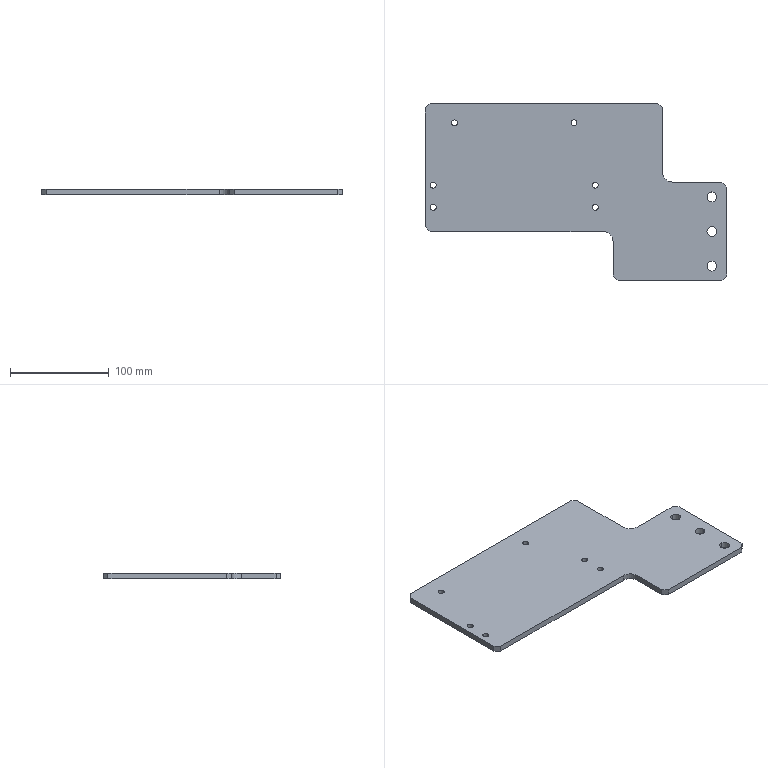Part | STEP file | J453-EBZ05-04-04-Part-1 | 1 solid | 36 faces | box 305 x 180 x 6 mm | volume 238576 mm3 | cylinder 20 | plane 16 | commonest cylinder face diameters 6 x12 10 x6 20 x2